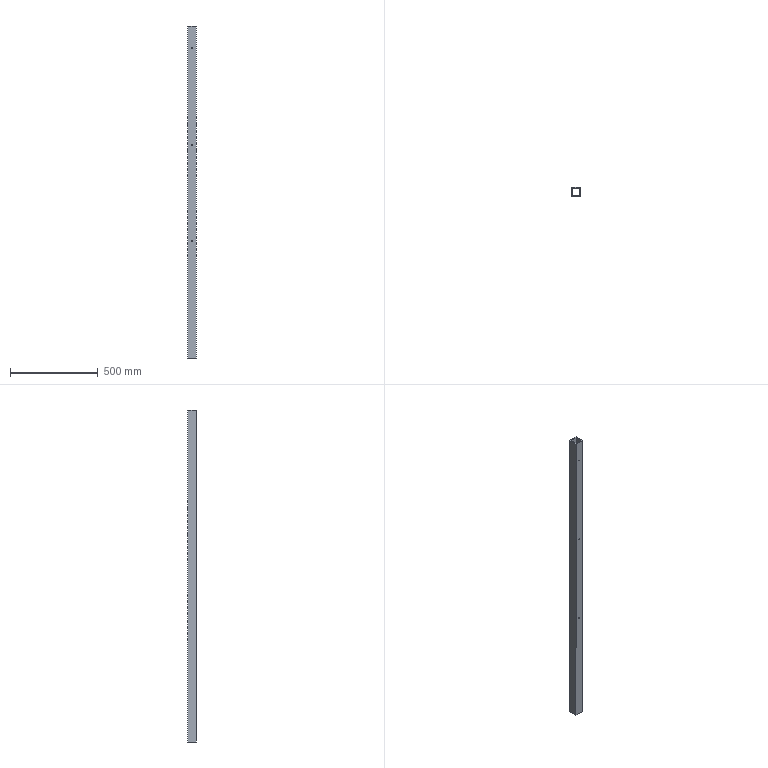Part | NX | features solid 2 | 1 solid | 16 faces | box 50 x 50 x 1896 mm | volume 1706083 mm3 | plane 10 | cylinder 6 | commonest cylinder face diameters 5.188 x6
STEP:
#1=CARTESIAN_POINT('',(-1085.,0.,62.406));
#2=VERTEX_POINT('',#1);
#3=CARTESIAN_POINT('',(-1085.,5.,62.406));
#4=VERTEX_POINT('',#3);
#5=CARTESIAN_POINT('',(-1085.,1859.345,62.406));
#6=DIRECTION('',(0.,-1.,0.));
#7=VECTOR('',#6,1000.);
#8=LINE('',#5,#7);
#9=EDGE_CURVE('',#2,#4,#8,.F.);
#10=ORIENTED_EDGE('',*,*,#9,.T.);
#11=CARTESIAN_POINT('',(-1085.,5.,67.594));
#12=VERTEX_POINT('',#11);
#13=CARTESIAN_POINT('',(-1085.,5.,65.));
#14=DIRECTION('',(0.,1.,0.));
#15=DIRECTION('',(0.,0.,-1.));
#16=AXIS2_PLACEMENT_3D('',#13,#14,#15);
#17=CIRCLE('',#16,2.594);
#18=EDGE_CURVE('',#4,#12,#17,.T.);
#19=ORIENTED_EDGE('',*,*,#18,.T.);
#20=CARTESIAN_POINT('',(-1085.,0.,67.594));
#21=VERTEX_POINT('',#20);
#22=CARTESIAN_POINT('',(-1085.,1859.345,67.594));
#23=DIRECTION('',(0.,-1.,0.));
#24=VECTOR('',#23,1000.);
#25=LINE('',#22,#24);
#26=EDGE_CURVE('',#12,#21,#25,.T.);
#27=ORIENTED_EDGE('',*,*,#26,.T.);
#28=CARTESIAN_POINT('',(-1085.,0.,65.));
#29=DIRECTION('',(0.,-1.,0.));
#30=DIRECTION('',(0.,0.,1.));
#31=AXIS2_PLACEMENT_3D('',#28,#29,#30);
#32=CIRCLE('',#31,2.594);
#33=EDGE_CURVE('',#21,#2,#32,.T.);
#34=ORIENTED_EDGE('',*,*,#33,.T.);
#35=EDGE_LOOP('',(#10,#19,#27,#34));
#36=FACE_BOUND('',#35,.T.);
#37=CARTESIAN_POINT('',(-1085.,1859.345,65.));
#38=DIRECTION('',(0.,-1.,0.));
#39=DIRECTION('',(0.,0.,1.));
#40=AXIS2_PLACEMENT_3D('',#37,#38,#39);
#41=CYLINDRICAL_SURFACE('',#40,2.594);
#42=ADVANCED_FACE('',(#36),#41,.F.);
#43=CARTESIAN_POINT('',(-1085.,0.,612.406));
#44=VERTEX_POINT('',#43);
#45=CARTESIAN_POINT('',(-1085.,5.,612.406));
#46=VERTEX_POINT('',#45);
#47=CARTESIAN_POINT('',(-1085.,1859.345,612.406));
#48=DIRECTION('',(0.,-1.,0.));
#49=VECTOR('',#48,1000.);
#50=LINE('',#47,#49);
#51=EDGE_CURVE('',#44,#46,#50,.F.);
#52=ORIENTED_EDGE('',*,*,#51,.T.);
#53=CARTESIAN_POINT('',(-1085.,5.,617.594));
#54=VERTEX_POINT('',#53);
#55=CARTESIAN_POINT('',(-1085.,5.,615.));
#56=DIRECTION('',(0.,1.,0.));
#57=DIRECTION('',(0.,0.,-1.));
#58=AXIS2_PLACEMENT_3D('',#55,#56,#57);
#59=CIRCLE('',#58,2.594);
#60=EDGE_CURVE('',#46,#54,#59,.T.);
#61=ORIENTED_EDGE('',*,*,#60,.T.);
#62=CARTESIAN_POINT('',(-1085.,0.,617.594));
#63=VERTEX_POINT('',#62);
#64=CARTESIAN_POINT('',(-1085.,1859.345,617.594));
#65=DIRECTION('',(0.,-1.,0.));
#66=VECTOR('',#65,1000.);
#67=LINE('',#64,#66);
#68=EDGE_CURVE('',#54,#63,#67,.T.);
#69=ORIENTED_EDGE('',*,*,#68,.T.);
#70=CARTESIAN_POINT('',(-1085.,0.,615.));
#71=DIRECTION('',(0.,-1.,0.));
#72=DIRECTION('',(0.,0.,1.));
#73=AXIS2_PLACEMENT_3D('',#70,#71,#72);
#74=CIRCLE('',#73,2.594);
#75=EDGE_CURVE('',#63,#44,#74,.T.);
#76=ORIENTED_EDGE('',*,*,#75,.T.);
#77=EDGE_LOOP('',(#52,#61,#69,#76));
#78=FACE_BOUND('',#77,.T.);
#79=CARTESIAN_POINT('',(-1085.,1859.345,615.));
#80=DIRECTION('',(0.,-1.,0.));
#81=DIRECTION('',(0.,0.,1.));
#82=AXIS2_PLACEMENT_3D('',#79,#80,#81);
#83=CYLINDRICAL_SURFACE('',#82,2.594);
#84=ADVANCED_FACE('',(#78),#83,.F.);
#85=CARTESIAN_POINT('',(-1085.,5.,1162.406));
#86=VERTEX_POINT('',#85);
#87=CARTESIAN_POINT('',(-1085.,0.,1162.406));
#88=VERTEX_POINT('',#87);
#89=CARTESIAN_POINT('',(-1085.,1859.345,1162.406));
#90=DIRECTION('',(0.,-1.,0.));
#91=VECTOR('',#90,1000.);
#92=LINE('',#89,#91);
#93=EDGE_CURVE('',#86,#88,#92,.T.);
#94=ORIENTED_EDGE('',*,*,#93,.F.);
#95=CARTESIAN_POINT('',(-1085.,5.,1167.594));
#96=VERTEX_POINT('',#95);
#97=CARTESIAN_POINT('',(-1085.,5.,1165.));
#98=DIRECTION('',(0.,1.,0.));
#99=DIRECTION('',(0.,0.,-1.));
#100=AXIS2_PLACEMENT_3D('',#97,#98,#99);
#101=CIRCLE('',#100,2.594);
#102=EDGE_CURVE('',#86,#96,#101,.T.);
#103=ORIENTED_EDGE('',*,*,#102,.T.);
#104=CARTESIAN_POINT('',(-1085.,0.,1167.594));
#105=VERTEX_POINT('',#104);
#106=CARTESIAN_POINT('',(-1085.,1859.345,1167.594));
#107=DIRECTION('',(0.,-1.,0.));
#108=VECTOR('',#107,1000.);
#109=LINE('',#106,#108);
#110=EDGE_CURVE('',#105,#96,#109,.F.);
#111=ORIENTED_EDGE('',*,*,#110,.F.);
#112=CARTESIAN_POINT('',(-1085.,0.,1165.));
#113=DIRECTION('',(0.,-1.,0.));
#114=DIRECTION('',(0.,0.,1.));
#115=AXIS2_PLACEMENT_3D('',#112,#113,#114);
#116=CIRCLE('',#115,2.594);
#117=EDGE_CURVE('',#105,#88,#116,.T.);
#118=ORIENTED_EDGE('',*,*,#117,.T.);
#119=EDGE_LOOP('',(#94,#103,#111,#118));
#120=FACE_BOUND('',#119,.T.);
#121=CARTESIAN_POINT('',(-1085.,1859.345,1165.));
#122=DIRECTION('',(0.,-1.,0.));
#123=DIRECTION('',(0.,0.,1.));
#124=AXIS2_PLACEMENT_3D('',#121,#122,#123);
#125=CYLINDRICAL_SURFACE('',#124,2.594);
#126=ADVANCED_FACE('',(#120),#125,.F.);
#127=CARTESIAN_POINT('',(-1110.,50.,-603.));
#128=VERTEX_POINT('',#127);
#129=CARTESIAN_POINT('',(-1110.,50.,1293.));
#130=VERTEX_POINT('',#129);
#131=CARTESIAN_POINT('',(-1110.,50.,-495.));
#132=DIRECTION('',(0.,0.,1.));
#133=VECTOR('',#132,1000.);
#134=LINE('',#131,#133);
#135=EDGE_CURVE('',#128,#130,#134,.T.);
#136=ORIENTED_EDGE('',*,*,#135,.T.);
#137=CARTESIAN_POINT('',(-1060.,50.,1293.));
#138=VERTEX_POINT('',#137);
#139=CARTESIAN_POINT('',(-1110.,50.,1293.));
#140=DIRECTION('',(-1.,0.,0.));
#141=VECTOR('',#140,1000.);
#142=LINE('',#139,#141);
#143=EDGE_CURVE('',#138,#130,#142,.T.);
#144=ORIENTED_EDGE('',*,*,#143,.F.);
#145=CARTESIAN_POINT('',(-1060.,50.,-603.));
#146=VERTEX_POINT('',#145);
#147=CARTESIAN_POINT('',(-1060.,50.,-495.));
#148=DIRECTION('',(0.,0.,-1.));
#149=VECTOR('',#148,1000.);
#150=LINE('',#147,#149);
#151=EDGE_CURVE('',#138,#146,#150,.T.);
#152=ORIENTED_EDGE('',*,*,#151,.T.);
#153=CARTESIAN_POINT('',(-1110.,50.,-603.));
#154=DIRECTION('',(-1.,0.,0.));
#155=VECTOR('',#154,1000.);
#156=LINE('',#153,#155);
#157=EDGE_CURVE('',#146,#128,#156,.T.);
#158=ORIENTED_EDGE('',*,*,#157,.T.);
#159=EDGE_LOOP('',(#136,#144,#152,#158));
#160=FACE_BOUND('',#159,.T.);
#161=CARTESIAN_POINT('',(-1110.,50.,-495.));
#162=DIRECTION('',(0.,-1.,0.));
#163=DIRECTION('',(-1.,0.,0.));
#164=AXIS2_PLACEMENT_3D('',#161,#162,#163);
#165=PLANE('',#164);
#166=ADVANCED_FACE('',(#160),#165,.F.);
#167=CARTESIAN_POINT('',(-1105.,45.,1293.));
#168=VERTEX_POINT('',#167);
#169=CARTESIAN_POINT('',(-1065.,45.,1293.));
#170=VERTEX_POINT('',#169);
#171=CARTESIAN_POINT('',(-1060.,45.,1293.));
#172=DIRECTION('',(1.,0.,0.));
#173=VECTOR('',#172,1000.);
#174=LINE('',#171,#173);
#175=EDGE_CURVE('',#168,#170,#174,.T.);
#176=ORIENTED_EDGE('',*,*,#175,.F.);
#177=CARTESIAN_POINT('',(-1105.,45.,-603.));
#178=VERTEX_POINT('',#177);
#179=CARTESIAN_POINT('',(-1105.,45.,-495.));
#180=DIRECTION('',(0.,0.,1.));
#181=VECTOR('',#180,1000.);
#182=LINE('',#179,#181);
#183=EDGE_CURVE('',#178,#168,#182,.T.);
#184=ORIENTED_EDGE('',*,*,#183,.F.);
#185=CARTESIAN_POINT('',(-1065.,45.,-603.));
#186=VERTEX_POINT('',#185);
#187=CARTESIAN_POINT('',(-1060.,45.,-603.));
#188=DIRECTION('',(1.,0.,0.));
#189=VECTOR('',#188,1000.);
#190=LINE('',#187,#189);
#191=EDGE_CURVE('',#178,#186,#190,.T.);
#192=ORIENTED_EDGE('',*,*,#191,.T.);
#193=CARTESIAN_POINT('',(-1065.,45.,-495.));
#194=DIRECTION('',(0.,0.,-1.));
#195=VECTOR('',#194,1000.);
#196=LINE('',#193,#195);
#197=EDGE_CURVE('',#170,#186,#196,.T.);
#198=ORIENTED_EDGE('',*,*,#197,.F.);
#199=EDGE_LOOP('',(#176,#184,#192,#198));
#200=FACE_BOUND('',#199,.T.);
#201=CARTESIAN_POINT('',(-1105.,45.,-495.));
#202=DIRECTION('',(0.,-1.,0.));
#203=DIRECTION('',(-1.,0.,0.));
#204=AXIS2_PLACEMENT_3D('',#201,#202,#203);
#205=PLANE('',#204);
#206=ADVANCED_FACE('',(#200),#205,.T.);
#207=CARTESIAN_POINT('',(-1110.,0.,-603.));
#208=VERTEX_POINT('',#207);
#209=CARTESIAN_POINT('',(-1110.,0.,1293.));
#210=VERTEX_POINT('',#209);
#211=CARTESIAN_POINT('',(-1110.,0.,1245.));
#212=DIRECTION('',(0.,0.,1.));
#213=VECTOR('',#212,1000.);
#214=LINE('',#211,#213);
#215=EDGE_CURVE('',#208,#210,#214,.T.);
#216=ORIENTED_EDGE('',*,*,#215,.T.);
#217=CARTESIAN_POINT('',(-1110.,0.,1293.));
#218=DIRECTION('',(0.,-1.,0.));
#219=VECTOR('',#218,1000.);
#220=LINE('',#217,#219);
#221=EDGE_CURVE('',#130,#210,#220,.T.);
#222=ORIENTED_EDGE('',*,*,#221,.F.);
#223=ORIENTED_EDGE('',*,*,#135,.F.);
#224=CARTESIAN_POINT('',(-1110.,0.,-603.));
#225=DIRECTION('',(0.,-1.,0.));
#226=VECTOR('',#225,1000.);
#227=LINE('',#224,#226);
#228=EDGE_CURVE('',#128,#208,#227,.T.);
#229=ORIENTED_EDGE('',*,*,#228,.T.);
#230=EDGE_LOOP('',(#216,#222,#223,#229));
#231=FACE_BOUND('',#230,.T.);
#232=CARTESIAN_POINT('',(-1110.,0.,1245.));
#233=DIRECTION('',(1.,0.,0.));
#234=DIRECTION('',(0.,-1.,0.));
#235=AXIS2_PLACEMENT_3D('',#232,#233,#234);
#236=PLANE('',#235);
#237=ADVANCED_FACE('',(#231),#236,.F.);
#238=ORIENTED_EDGE('',*,*,#151,.F.);
#239=CARTESIAN_POINT('',(-1060.,0.,1293.));
#240=VERTEX_POINT('',#239);
#241=CARTESIAN_POINT('',(-1060.,0.,1293.));
#242=DIRECTION('',(0.,1.,0.));
#243=VECTOR('',#242,1000.);
#244=LINE('',#241,#243);
#245=EDGE_CURVE('',#240,#138,#244,.T.);
#246=ORIENTED_EDGE('',*,*,#245,.F.);
#247=CARTESIAN_POINT('',(-1060.,0.,-603.));
#248=VERTEX_POINT('',#247);
#249=CARTESIAN_POINT('',(-1060.,0.,-495.));
#250=DIRECTION('',(0.,0.,-1.));
#251=VECTOR('',#250,1000.);
#252=LINE('',#249,#251);
#253=EDGE_CURVE('',#240,#248,#252,.T.);
#254=ORIENTED_EDGE('',*,*,#253,.T.);
#255=CARTESIAN_POINT('',(-1060.,0.,-603.));
#256=DIRECTION('',(0.,1.,0.));
#257=VECTOR('',#256,1000.);
#258=LINE('',#255,#257);
#259=EDGE_CURVE('',#248,#146,#258,.T.);
#260=ORIENTED_EDGE('',*,*,#259,.T.);
#261=EDGE_LOOP('',(#238,#246,#254,#260));
#262=FACE_BOUND('',#261,.T.);
#263=CARTESIAN_POINT('',(-1060.,0.,-495.));
#264=DIRECTION('',(-1.,0.,0.));
#265=DIRECTION('',(0.,0.,1.));
#266=AXIS2_PLACEMENT_3D('',#263,#264,#265);
#267=PLANE('',#266);
#268=ADVANCED_FACE('',(#262),#267,.F.);
#269=CARTESIAN_POINT('',(-1065.,5.,-603.));
#270=VERTEX_POINT('',#269);
#271=CARTESIAN_POINT('',(-1065.,0.,-603.));
#272=DIRECTION('',(0.,-1.,0.));
#273=VECTOR('',#272,1000.);
#274=LINE('',#271,#273);
#275=EDGE_CURVE('',#186,#270,#274,.T.);
#276=ORIENTED_EDGE('',*,*,#275,.F.);
#277=ORIENTED_EDGE('',*,*,#191,.F.);
#278=CARTESIAN_POINT('',(-1105.,5.,-603.));
#279=VERTEX_POINT('',#278);
#280=CARTESIAN_POINT('',(-1105.,0.,-603.));
#281=DIRECTION('',(0.,1.,0.));
#282=VECTOR('',#281,1000.);
#283=LINE('',#280,#282);
#284=EDGE_CURVE('',#279,#178,#283,.T.);
#285=ORIENTED_EDGE('',*,*,#284,.F.);
#286=CARTESIAN_POINT('',(-1060.,5.,-603.));
#287=DIRECTION('',(-1.,0.,0.));
#288=VECTOR('',#287,1000.);
#289=LINE('',#286,#288);
#290=EDGE_CURVE('',#270,#279,#289,.T.);
#291=ORIENTED_EDGE('',*,*,#290,.F.);
#292=EDGE_LOOP('',(#276,#277,#285,#291));
#293=FACE_BOUND('',#292,.T.);
#294=ORIENTED_EDGE('',*,*,#228,.F.);
#295=ORIENTED_EDGE('',*,*,#157,.F.);
#296=ORIENTED_EDGE('',*,*,#259,.F.);
#297=CARTESIAN_POINT('',(-1060.,0.,-603.));
#298=DIRECTION('',(-1.,0.,0.));
#299=VECTOR('',#298,1000.);
#300=LINE('',#297,#299);
#301=EDGE_CURVE('',#248,#208,#300,.T.);
#302=ORIENTED_EDGE('',*,*,#301,.T.);
#303=EDGE_LOOP('',(#294,#295,#296,#302));
#304=FACE_BOUND('',#303,.T.);
#305=CARTESIAN_POINT('',(-1060.,0.,-603.));
#306=DIRECTION('',(0.,0.,1.));
#307=DIRECTION('',(0.,-1.,0.));
#308=AXIS2_PLACEMENT_3D('',#305,#306,#307);
#309=PLANE('',#308);
#310=ADVANCED_FACE('',(#293,#304),#309,.F.);
#311=CARTESIAN_POINT('',(-1105.,5.,1293.));
#312=VERTEX_POINT('',#311);
#313=CARTESIAN_POINT('',(-1105.,0.,1293.));
#314=DIRECTION('',(0.,1.,0.));
#315=VECTOR('',#314,1000.);
#316=LINE('',#313,#315);
#317=EDGE_CURVE('',#312,#168,#316,.T.);
#318=ORIENTED_EDGE('',*,*,#317,.F.);
#319=CARTESIAN_POINT('',(-1105.,5.,1245.));
#320=DIRECTION('',(0.,0.,1.));
#321=VECTOR('',#320,1000.);
#322=LINE('',#319,#321);
#323=EDGE_CURVE('',#279,#312,#322,.T.);
#324=ORIENTED_EDGE('',*,*,#323,.F.);
#325=ORIENTED_EDGE('',*,*,#284,.T.);
#326=ORIENTED_EDGE('',*,*,#183,.T.);
#327=EDGE_LOOP('',(#318,#324,#325,#326));
#328=FACE_BOUND('',#327,.T.);
#329=CARTESIAN_POINT('',(-1105.,5.,1245.));
#330=DIRECTION('',(1.,0.,0.));
#331=DIRECTION('',(0.,-1.,0.));
#332=AXIS2_PLACEMENT_3D('',#329,#330,#331);
#333=PLANE('',#332);
#334=ADVANCED_FACE('',(#328),#333,.T.);
#335=ORIENTED_EDGE('',*,*,#317,.T.);
#336=ORIENTED_EDGE('',*,*,#175,.T.);
#337=CARTESIAN_POINT('',(-1065.,5.,1293.));
#338=VERTEX_POINT('',#337);
#339=CARTESIAN_POINT('',(-1065.,45.,1293.));
#340=DIRECTION('',(0.,1.,0.));
#341=VECTOR('',#340,1000.);
#342=LINE('',#339,#341);
#343=EDGE_CURVE('',#338,#170,#342,.T.);
#344=ORIENTED_EDGE('',*,*,#343,.F.);
#345=CARTESIAN_POINT('',(-1065.,5.,1293.));
#346=DIRECTION('',(1.,0.,0.));
#347=VECTOR('',#346,1000.);
#348=LINE('',#345,#347);
#349=EDGE_CURVE('',#312,#338,#348,.T.);
#350=ORIENTED_EDGE('',*,*,#349,.F.);
#351=EDGE_LOOP('',(#335,#336,#344,#350));
#352=FACE_BOUND('',#351,.T.);
#353=ORIENTED_EDGE('',*,*,#143,.T.);
#354=ORIENTED_EDGE('',*,*,#221,.T.);
#355=CARTESIAN_POINT('',(-1060.,0.,1293.));
#356=DIRECTION('',(1.,0.,0.));
#357=VECTOR('',#356,1000.);
#358=LINE('',#355,#357);
#359=EDGE_CURVE('',#210,#240,#358,.T.);
#360=ORIENTED_EDGE('',*,*,#359,.T.);
#361=ORIENTED_EDGE('',*,*,#245,.T.);
#362=EDGE_LOOP('',(#353,#354,#360,#361));
#363=FACE_BOUND('',#362,.T.);
#364=CARTESIAN_POINT('',(-1060.,0.,1293.));
#365=DIRECTION('',(0.,0.,1.));
#366=DIRECTION('',(0.,-1.,0.));
#367=AXIS2_PLACEMENT_3D('',#364,#365,#366);
#368=PLANE('',#367);
#369=ADVANCED_FACE('',(#352,#363),#368,.T.);
#370=ORIENTED_EDGE('',*,*,#343,.T.);
#371=ORIENTED_EDGE('',*,*,#197,.T.);
#372=ORIENTED_EDGE('',*,*,#275,.T.);
#373=CARTESIAN_POINT('',(-1065.,5.,-495.));
#374=DIRECTION('',(0.,0.,-1.));
#375=VECTOR('',#374,1000.);
#376=LINE('',#373,#375);
#377=EDGE_CURVE('',#338,#270,#376,.T.);
#378=ORIENTED_EDGE('',*,*,#377,.F.);
#379=EDGE_LOOP('',(#370,#371,#372,#378));
#380=FACE_BOUND('',#379,.T.);
#381=CARTESIAN_POINT('',(-1065.,45.,-495.));
#382=DIRECTION('',(-1.,0.,0.));
#383=DIRECTION('',(0.,0.,1.));
#384=AXIS2_PLACEMENT_3D('',#381,#382,#383);
#385=PLANE('',#384);
#386=ADVANCED_FACE('',(#380),#385,.T.);
#387=ORIENTED_EDGE('',*,*,#117,.F.);
#388=CARTESIAN_POINT('',(-1085.,0.,1165.));
#389=DIRECTION('',(0.,-1.,0.));
#390=DIRECTION('',(0.,0.,1.));
#391=AXIS2_PLACEMENT_3D('',#388,#389,#390);
#392=CIRCLE('',#391,2.594);
#393=EDGE_CURVE('',#88,#105,#392,.T.);
#394=ORIENTED_EDGE('',*,*,#393,.F.);
#395=EDGE_LOOP('',(#387,#394));
#396=FACE_BOUND('',#395,.T.);
#397=ORIENTED_EDGE('',*,*,#75,.F.);
#398=CARTESIAN_POINT('',(-1085.,0.,615.));
#399=DIRECTION('',(0.,-1.,0.));
#400=DIRECTION('',(0.,0.,1.));
#401=AXIS2_PLACEMENT_3D('',#398,#399,#400);
#402=CIRCLE('',#401,2.594);
#403=EDGE_CURVE('',#44,#63,#402,.T.);
#404=ORIENTED_EDGE('',*,*,#403,.F.);
#405=EDGE_LOOP('',(#397,#404));
#406=FACE_BOUND('',#405,.T.);
#407=ORIENTED_EDGE('',*,*,#33,.F.);
#408=CARTESIAN_POINT('',(-1085.,0.,65.));
#409=DIRECTION('',(0.,-1.,0.));
#410=DIRECTION('',(0.,0.,1.));
#411=AXIS2_PLACEMENT_3D('',#408,#409,#410);
#412=CIRCLE('',#411,2.594);
#413=EDGE_CURVE('',#2,#21,#412,.T.);
#414=ORIENTED_EDGE('',*,*,#413,.F.);
#415=EDGE_LOOP('',(#407,#414));
#416=FACE_BOUND('',#415,.T.);
#417=ORIENTED_EDGE('',*,*,#253,.F.);
#418=ORIENTED_EDGE('',*,*,#359,.F.);
#419=ORIENTED_EDGE('',*,*,#215,.F.);
#420=ORIENTED_EDGE('',*,*,#301,.F.);
#421=EDGE_LOOP('',(#417,#418,#419,#420));
#422=FACE_BOUND('',#421,.T.);
#423=CARTESIAN_POINT('',(-1060.,0.,-495.));
#424=DIRECTION('',(0.,1.,0.));
#425=DIRECTION('',(1.,0.,0.));
#426=AXIS2_PLACEMENT_3D('',#423,#424,#425);
#427=PLANE('',#426);
#428=ADVANCED_FACE('',(#396,#406,#416,#422),#427,.F.);
#429=CARTESIAN_POINT('',(-1085.,5.,1165.));
#430=DIRECTION('',(0.,1.,0.));
#431=DIRECTION('',(0.,0.,-1.));
#432=AXIS2_PLACEMENT_3D('',#429,#430,#431);
#433=CIRCLE('',#432,2.594);
#434=EDGE_CURVE('',#96,#86,#433,.T.);
#435=ORIENTED_EDGE('',*,*,#434,.F.);
#436=ORIENTED_EDGE('',*,*,#102,.F.);
#437=EDGE_LOOP('',(#435,#436));
#438=FACE_BOUND('',#437,.T.);
#439=CARTESIAN_POINT('',(-1085.,5.,615.));
#440=DIRECTION('',(0.,1.,0.));
#441=DIRECTION('',(0.,0.,-1.));
#442=AXIS2_PLACEMENT_3D('',#439,#440,#441);
#443=CIRCLE('',#442,2.594);
#444=EDGE_CURVE('',#54,#46,#443,.T.);
#445=ORIENTED_EDGE('',*,*,#444,.F.);
#446=ORIENTED_EDGE('',*,*,#60,.F.);
#447=EDGE_LOOP('',(#445,#446));
#448=FACE_BOUND('',#447,.T.);
#449=CARTESIAN_POINT('',(-1085.,5.,65.));
#450=DIRECTION('',(0.,1.,0.));
#451=DIRECTION('',(0.,0.,-1.));
#452=AXIS2_PLACEMENT_3D('',#449,#450,#451);
#453=CIRCLE('',#452,2.594);
#454=EDGE_CURVE('',#12,#4,#453,.T.);
#455=ORIENTED_EDGE('',*,*,#454,.F.);
#456=ORIENTED_EDGE('',*,*,#18,.F.);
#457=EDGE_LOOP('',(#455,#456));
#458=FACE_BOUND('',#457,.T.);
#459=ORIENTED_EDGE('',*,*,#349,.T.);
#460=ORIENTED_EDGE('',*,*,#377,.T.);
#461=ORIENTED_EDGE('',*,*,#290,.T.);
#462=ORIENTED_EDGE('',*,*,#323,.T.);
#463=EDGE_LOOP('',(#459,#460,#461,#462));
#464=FACE_BOUND('',#463,.T.);
#465=CARTESIAN_POINT('',(-1065.,5.,1245.));
#466=DIRECTION('',(0.,1.,0.));
#467=DIRECTION('',(1.,0.,0.));
#468=AXIS2_PLACEMENT_3D('',#465,#466,#467);
#469=PLANE('',#468);
#470=ADVANCED_FACE('',(#438,#448,#458,#464),#469,.T.);
#471=ORIENTED_EDGE('',*,*,#434,.T.);
#472=ORIENTED_EDGE('',*,*,#93,.T.);
#473=ORIENTED_EDGE('',*,*,#393,.T.);
#474=ORIENTED_EDGE('',*,*,#110,.T.);
#475=EDGE_LOOP('',(#471,#472,#473,#474));
#476=FACE_BOUND('',#475,.T.);
#477=CARTESIAN_POINT('',(-1085.,1859.345,1165.));
#478=DIRECTION('',(0.,-1.,0.));
#479=DIRECTION('',(0.,0.,1.));
#480=AXIS2_PLACEMENT_3D('',#477,#478,#479);
#481=CYLINDRICAL_SURFACE('',#480,2.594);
#482=ADVANCED_FACE('',(#476),#481,.F.);
#483=ORIENTED_EDGE('',*,*,#444,.T.);
#484=ORIENTED_EDGE('',*,*,#51,.F.);
#485=ORIENTED_EDGE('',*,*,#403,.T.);
#486=ORIENTED_EDGE('',*,*,#68,.F.);
#487=EDGE_LOOP('',(#483,#484,#485,#486));
#488=FACE_BOUND('',#487,.T.);
#489=CARTESIAN_POINT('',(-1085.,1859.345,615.));
#490=DIRECTION('',(0.,-1.,0.));
#491=DIRECTION('',(0.,0.,1.));
#492=AXIS2_PLACEMENT_3D('',#489,#490,#491);
#493=CYLINDRICAL_SURFACE('',#492,2.594);
#494=ADVANCED_FACE('',(#488),#493,.F.);
#495=ORIENTED_EDGE('',*,*,#454,.T.);
#496=ORIENTED_EDGE('',*,*,#9,.F.);
#497=ORIENTED_EDGE('',*,*,#413,.T.);
#498=ORIENTED_EDGE('',*,*,#26,.F.);
#499=EDGE_LOOP('',(#495,#496,#497,#498));
#500=FACE_BOUND('',#499,.T.);
#501=CARTESIAN_POINT('',(-1085.,1859.345,65.));
#502=DIRECTION('',(0.,-1.,0.));
#503=DIRECTION('',(0.,0.,1.));
#504=AXIS2_PLACEMENT_3D('',#501,#502,#503);
#505=CYLINDRICAL_SURFACE('',#504,2.594);
#506=ADVANCED_FACE('',(#500),#505,.F.);
#507=CLOSED_SHELL('',(#42,#84,#126,#166,#206,#237,#268,#310,#334,#369,#386,#428,#470,#482,#494,#506));
#508=MANIFOLD_SOLID_BREP('',#507);
#509=(LENGTH_UNIT()NAMED_UNIT(*)SI_UNIT(.MILLI.,.METRE.));
#510=UNCERTAINTY_MEASURE_WITH_UNIT(LENGTH_MEASURE(0.00001),#509,'','');
#511=(NAMED_UNIT(*)PLANE_ANGLE_UNIT()SI_UNIT($,.RADIAN.));
#512=(NAMED_UNIT(*)SI_UNIT($,.STERADIAN.)SOLID_ANGLE_UNIT());
#513=(GEOMETRIC_REPRESENTATION_CONTEXT(3)GLOBAL_UNCERTAINTY_ASSIGNED_CONTEXT((#510))GLOBAL_UNIT_ASSIGNED_CONTEXT((#509,#511,#512))REPRESENTATION_CONTEXT('',''));
#514=ADVANCED_BREP_SHAPE_REPRESENTATION('',(#508),#513);